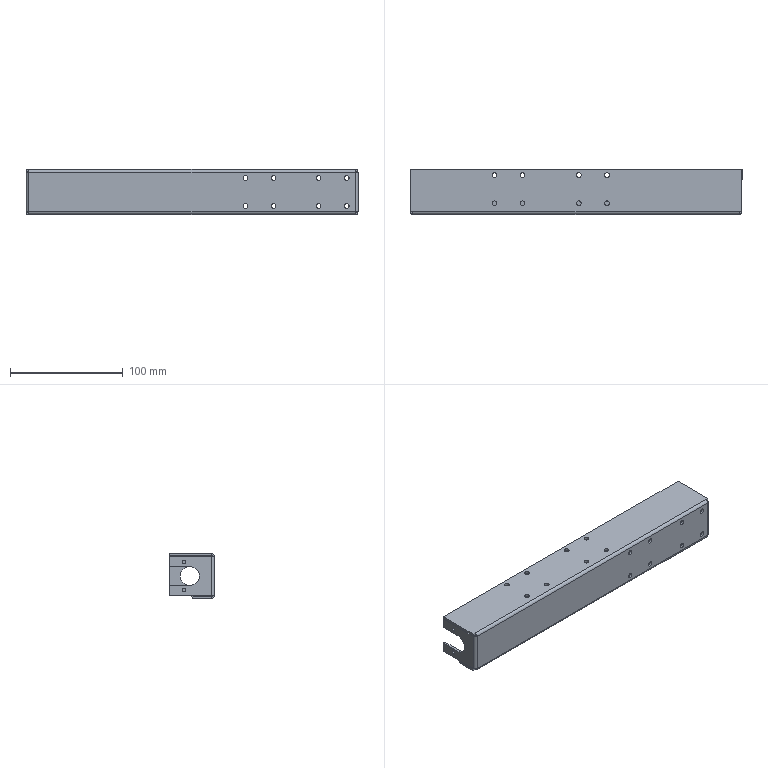Part | SolidWorks | features HoleWzd 3, EdgeFlange 2, ICE 2, FlatPattern 1, MoveFace 1, SMBaseFlange 1, SheetMetal 1 | 1 solid | 85 faces | box 295 x 40 x 40 mm | volume 59293 mm3 | cylinder 48 | plane 37 | commonest cylinder face diameters 4.2 x32 1 x4 3.3 x4 5 x4 17 x4